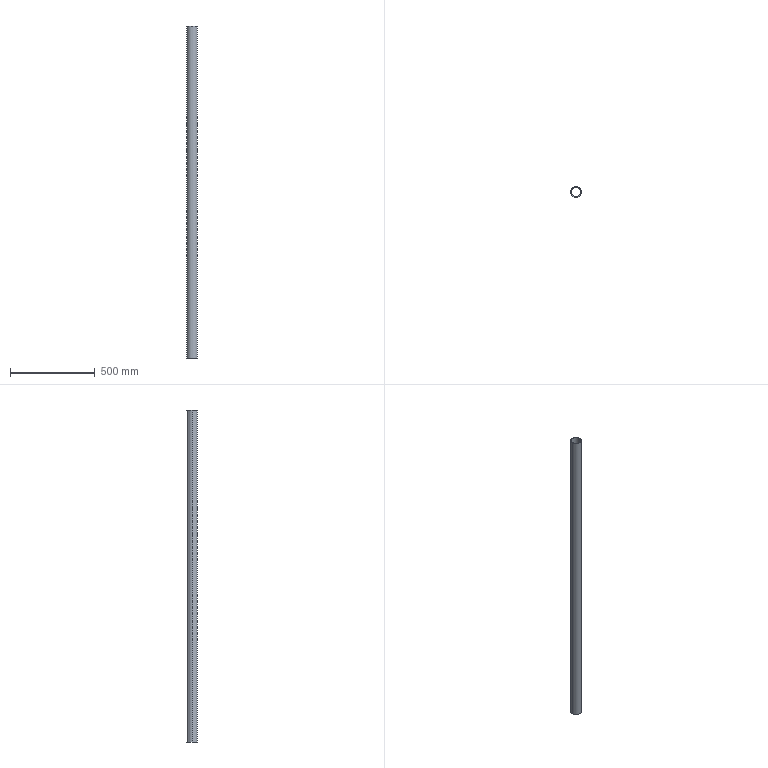Part | SolidWorks | features Extrusion 1, Shell 1 | 1 solid | 6 faces | box 63.5 x 63.5 x 1964 mm | volume 1190580 mm3 | cylinder 4 | plane 2 | commonest cylinder face diameters 57.1 x2 63.5 x2
STEP:
#1=CARTESIAN_POINT('',(-28.55,0.,1964.));
#2=VERTEX_POINT('',#1);
#3=CARTESIAN_POINT('',(28.55,0.,1964.));
#4=VERTEX_POINT('',#3);
#5=CARTESIAN_POINT('',(0.,0.,1964.));
#6=DIRECTION('',(0.,0.,1.));
#7=DIRECTION('',(1.,0.,0.));
#8=AXIS2_PLACEMENT_3D('',#5,#6,#7);
#9=CIRCLE('',#8,28.55);
#10=EDGE_CURVE('',#2,#4,#9,.T.);
#11=ORIENTED_EDGE('',*,*,#10,.T.);
#12=CARTESIAN_POINT('',(28.55,0.,0.));
#13=VERTEX_POINT('',#12);
#14=CARTESIAN_POINT('',(28.55,0.,1964.));
#15=DIRECTION('',(0.,0.,-1.));
#16=VECTOR('',#15,1000.);
#17=LINE('',#14,#16);
#18=EDGE_CURVE('',#4,#13,#17,.T.);
#19=ORIENTED_EDGE('',*,*,#18,.T.);
#20=CARTESIAN_POINT('',(-28.55,0.,0.));
#21=VERTEX_POINT('',#20);
#22=CARTESIAN_POINT('',(0.,0.,0.));
#23=DIRECTION('',(0.,0.,1.));
#24=DIRECTION('',(1.,0.,0.));
#25=AXIS2_PLACEMENT_3D('',#22,#23,#24);
#26=CIRCLE('',#25,28.55);
#27=EDGE_CURVE('',#21,#13,#26,.T.);
#28=ORIENTED_EDGE('',*,*,#27,.F.);
#29=CARTESIAN_POINT('',(-28.55,0.,1964.));
#30=DIRECTION('',(0.,0.,-1.));
#31=VECTOR('',#30,1000.);
#32=LINE('',#29,#31);
#33=EDGE_CURVE('',#2,#21,#32,.T.);
#34=ORIENTED_EDGE('',*,*,#33,.F.);
#35=EDGE_LOOP('',(#11,#19,#28,#34));
#36=FACE_OUTER_BOUND('',#35,.T.);
#37=CARTESIAN_POINT('',(0.,0.,1964.));
#38=DIRECTION('',(0.,0.,-1.));
#39=DIRECTION('',(-1.,0.,0.));
#40=AXIS2_PLACEMENT_3D('',#37,#38,#39);
#41=CYLINDRICAL_SURFACE('',#40,28.55);
#42=ADVANCED_FACE('',(#36),#41,.F.);
#43=CARTESIAN_POINT('',(31.75,0.,1964.));
#44=VERTEX_POINT('',#43);
#45=CARTESIAN_POINT('',(-31.75,0.,1964.));
#46=VERTEX_POINT('',#45);
#47=CARTESIAN_POINT('',(0.,0.,1964.));
#48=DIRECTION('',(0.,0.,1.));
#49=DIRECTION('',(1.,0.,0.));
#50=AXIS2_PLACEMENT_3D('',#47,#48,#49);
#51=CIRCLE('',#50,31.75);
#52=EDGE_CURVE('',#44,#46,#51,.T.);
#53=ORIENTED_EDGE('',*,*,#52,.F.);
#54=CARTESIAN_POINT('',(31.75,0.,0.));
#55=VERTEX_POINT('',#54);
#56=CARTESIAN_POINT('',(31.75,0.,1964.));
#57=DIRECTION('',(0.,0.,-1.));
#58=VECTOR('',#57,1000.);
#59=LINE('',#56,#58);
#60=EDGE_CURVE('',#44,#55,#59,.T.);
#61=ORIENTED_EDGE('',*,*,#60,.T.);
#62=CARTESIAN_POINT('',(-31.75,0.,0.));
#63=VERTEX_POINT('',#62);
#64=CARTESIAN_POINT('',(0.,0.,0.));
#65=DIRECTION('',(0.,0.,1.));
#66=DIRECTION('',(1.,0.,0.));
#67=AXIS2_PLACEMENT_3D('',#64,#65,#66);
#68=CIRCLE('',#67,31.75);
#69=EDGE_CURVE('',#55,#63,#68,.T.);
#70=ORIENTED_EDGE('',*,*,#69,.T.);
#71=CARTESIAN_POINT('',(-31.75,0.,1964.));
#72=DIRECTION('',(0.,0.,-1.));
#73=VECTOR('',#72,1000.);
#74=LINE('',#71,#73);
#75=EDGE_CURVE('',#46,#63,#74,.T.);
#76=ORIENTED_EDGE('',*,*,#75,.F.);
#77=EDGE_LOOP('',(#53,#61,#70,#76));
#78=FACE_OUTER_BOUND('',#77,.T.);
#79=CARTESIAN_POINT('',(0.,0.,1964.));
#80=DIRECTION('',(0.,0.,-1.));
#81=DIRECTION('',(-1.,0.,0.));
#82=AXIS2_PLACEMENT_3D('',#79,#80,#81);
#83=CYLINDRICAL_SURFACE('',#82,31.75);
#84=ADVANCED_FACE('',(#78),#83,.T.);
#85=ORIENTED_EDGE('',*,*,#60,.F.);
#86=CARTESIAN_POINT('',(0.,0.,1964.));
#87=DIRECTION('',(0.,0.,1.));
#88=DIRECTION('',(1.,0.,0.));
#89=AXIS2_PLACEMENT_3D('',#86,#87,#88);
#90=CIRCLE('',#89,31.75);
#91=EDGE_CURVE('',#46,#44,#90,.T.);
#92=ORIENTED_EDGE('',*,*,#91,.F.);
#93=ORIENTED_EDGE('',*,*,#75,.T.);
#94=CARTESIAN_POINT('',(0.,0.,0.));
#95=DIRECTION('',(0.,0.,1.));
#96=DIRECTION('',(1.,0.,0.));
#97=AXIS2_PLACEMENT_3D('',#94,#95,#96);
#98=CIRCLE('',#97,31.75);
#99=EDGE_CURVE('',#63,#55,#98,.T.);
#100=ORIENTED_EDGE('',*,*,#99,.T.);
#101=EDGE_LOOP('',(#85,#92,#93,#100));
#102=FACE_OUTER_BOUND('',#101,.T.);
#103=CARTESIAN_POINT('',(0.,0.,1964.));
#104=DIRECTION('',(0.,0.,-1.));
#105=DIRECTION('',(-1.,0.,0.));
#106=AXIS2_PLACEMENT_3D('',#103,#104,#105);
#107=CYLINDRICAL_SURFACE('',#106,31.75);
#108=ADVANCED_FACE('',(#102),#107,.T.);
#109=ORIENTED_EDGE('',*,*,#10,.F.);
#110=CARTESIAN_POINT('',(0.,0.,1964.));
#111=DIRECTION('',(0.,0.,1.));
#112=DIRECTION('',(1.,0.,0.));
#113=AXIS2_PLACEMENT_3D('',#110,#111,#112);
#114=CIRCLE('',#113,28.55);
#115=EDGE_CURVE('',#4,#2,#114,.T.);
#116=ORIENTED_EDGE('',*,*,#115,.F.);
#117=EDGE_LOOP('',(#109,#116));
#118=FACE_BOUND('',#117,.T.);
#119=ORIENTED_EDGE('',*,*,#91,.T.);
#120=ORIENTED_EDGE('',*,*,#52,.T.);
#121=EDGE_LOOP('',(#119,#120));
#122=FACE_OUTER_BOUND('',#121,.T.);
#123=CARTESIAN_POINT('',(0.,0.,1964.));
#124=DIRECTION('',(0.,0.,1.));
#125=DIRECTION('',(1.,0.,0.));
#126=AXIS2_PLACEMENT_3D('',#123,#124,#125);
#127=PLANE('',#126);
#128=ADVANCED_FACE('',(#118,#122),#127,.T.);
#129=ORIENTED_EDGE('',*,*,#27,.T.);
#130=CARTESIAN_POINT('',(0.,0.,0.));
#131=DIRECTION('',(0.,0.,1.));
#132=DIRECTION('',(1.,0.,0.));
#133=AXIS2_PLACEMENT_3D('',#130,#131,#132);
#134=CIRCLE('',#133,28.55);
#135=EDGE_CURVE('',#13,#21,#134,.T.);
#136=ORIENTED_EDGE('',*,*,#135,.T.);
#137=EDGE_LOOP('',(#129,#136));
#138=FACE_BOUND('',#137,.T.);
#139=ORIENTED_EDGE('',*,*,#99,.F.);
#140=ORIENTED_EDGE('',*,*,#69,.F.);
#141=EDGE_LOOP('',(#139,#140));
#142=FACE_OUTER_BOUND('',#141,.T.);
#143=CARTESIAN_POINT('',(0.,0.,0.));
#144=DIRECTION('',(0.,0.,1.));
#145=DIRECTION('',(1.,0.,0.));
#146=AXIS2_PLACEMENT_3D('',#143,#144,#145);
#147=PLANE('',#146);
#148=ADVANCED_FACE('',(#138,#142),#147,.F.);
#149=ORIENTED_EDGE('',*,*,#18,.F.);
#150=ORIENTED_EDGE('',*,*,#115,.T.);
#151=ORIENTED_EDGE('',*,*,#33,.T.);
#152=ORIENTED_EDGE('',*,*,#135,.F.);
#153=EDGE_LOOP('',(#149,#150,#151,#152));
#154=FACE_OUTER_BOUND('',#153,.T.);
#155=CARTESIAN_POINT('',(0.,0.,1964.));
#156=DIRECTION('',(0.,0.,-1.));
#157=DIRECTION('',(-1.,0.,0.));
#158=AXIS2_PLACEMENT_3D('',#155,#156,#157);
#159=CYLINDRICAL_SURFACE('',#158,28.55);
#160=ADVANCED_FACE('',(#154),#159,.F.);
#161=CLOSED_SHELL('',(#42,#84,#108,#128,#148,#160));
#162=MANIFOLD_SOLID_BREP('',#161);
#163=CARTESIAN_POINT('',(0.,0.,0.));
#164=DIRECTION('',(0.,0.,1.));
#165=DIRECTION('',(1.,0.,0.));
#166=AXIS2_PLACEMENT_3D('',#163,#164,#165);
#167=(LENGTH_UNIT()NAMED_UNIT(*)SI_UNIT(.MILLI.,.METRE.));
#168=UNCERTAINTY_MEASURE_WITH_UNIT(LENGTH_MEASURE(0.00001),#167,'','');
#169=(NAMED_UNIT(*)PLANE_ANGLE_UNIT()SI_UNIT($,.RADIAN.));
#170=(NAMED_UNIT(*)SI_UNIT($,.STERADIAN.)SOLID_ANGLE_UNIT());
#171=(GEOMETRIC_REPRESENTATION_CONTEXT(3)GLOBAL_UNCERTAINTY_ASSIGNED_CONTEXT((#168))GLOBAL_UNIT_ASSIGNED_CONTEXT((#167,#169,#170))REPRESENTATION_CONTEXT('',''));
#172=ADVANCED_BREP_SHAPE_REPRESENTATION('',(#162,#166),#171);